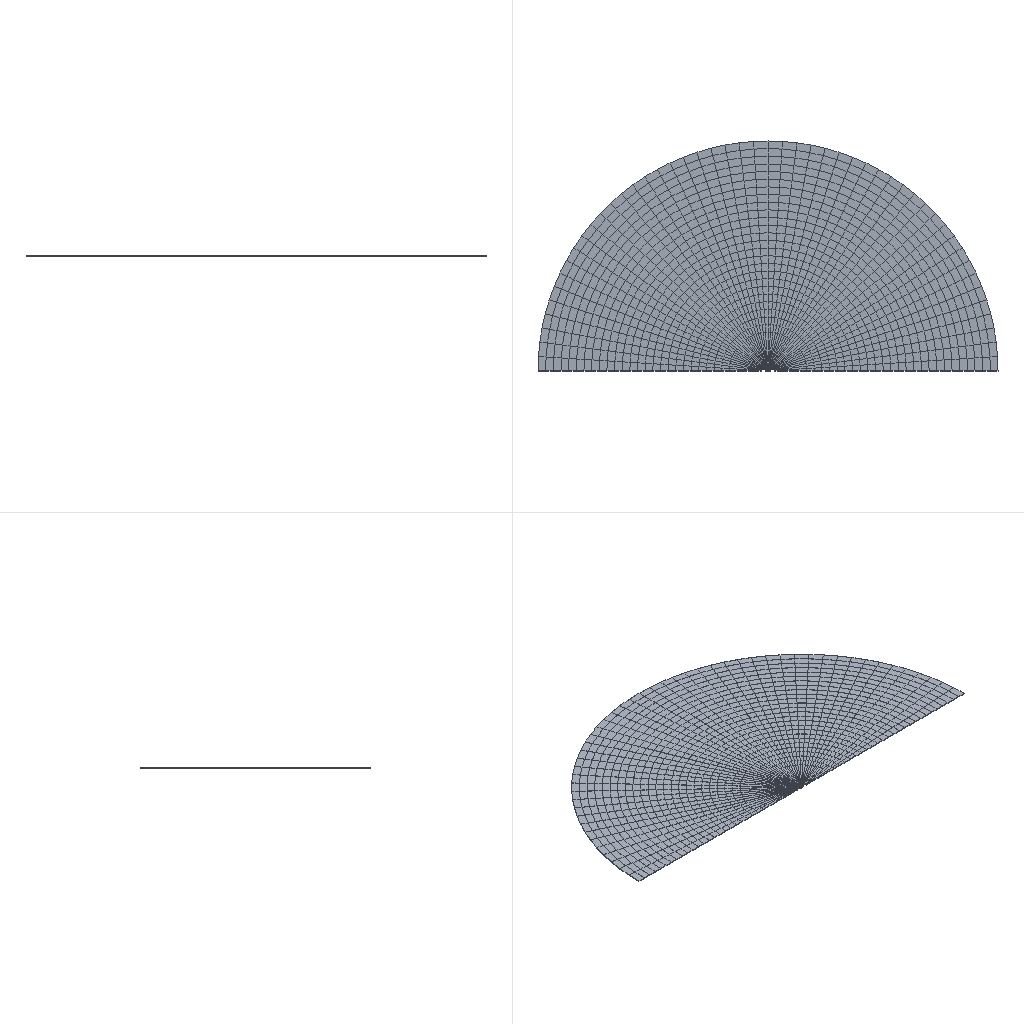Simulation study | abaqus
Set-up summary:
category,name,step,type,value,unit,region
solver,abaqus
solver,version,,,Abaqus/Standard 2020
units,not stated in the deck,,not stated
analysis,deck,,soils,soils
load_step,Step-1,Step-1,soils,nlgeom=True
contact,interactions,,,general=0 pairs=0 ties=0
load_step,requested,,,1
mesh,nodes,,,4272
mesh,elements,,,2036
element_type,C3D8PT,,solid,2036
load,load commands in deck,,count,3
bc,support commands in deck,,count,11
material,MATERIAL-1,,in results
check,setup vs results,,match,"per instance, exact: element labels, types and connectivity; labels of the nodes the elements use; coordinates of those nodes at SINGLE_PRECISION in 1 of 1 instance(s)"
Abaqus input file, long lists of numbers shortened:
*Heading
** Job name: Job-1 Model name: Model-1-30tian-1fenxibu
** Generated by: Abaqus/CAE 2020
*Preprint, echo=NO, model=NO, history=NO, contact=NO
**
** PARTS
**
*Part, name=Part-1
*Node
      1,   3.104,           0., 0.01
      2,   3.104,           0.,           0.
** (4270 more lines like these left out)
*Element, type=C3D8PT
   1,  226,  276, 1867,  495,    1,    2,   17,   72
   2,  495, 1867, 1868,  496,   72,   17,   18,   71
** (2034 more lines like these left out)
*Nset, nset=_PickedSet5, internal, generate
    1,  4272,     1
*Elset, elset=_PickedSet5, internal, generate
    1,  2036,     1
** Section: Section-1
*Solid Section, elset=_PickedSet5, material=Material-1
,
*End Part
**
**
** ASSEMBLY
**
*Assembly, name=Assembly
**
*Instance, name=Part-1-1, part=Part-1
         -3.,           0.,           0.
*End Instance
**
*Nset, nset=Set-re, instance=Part-1-1
 377, 378, 379, 380, 381, 382, 383, 384, 385, 386, 387, 388, 389, 390, 391, 392
 393, 394, 395, 396, 397, 398, 399, 400, 401, 402, 403, 404, 405, 414, 415, 416
** (2 more lines like these left out)
*Nset, nset=UPandBOTTOM, instance=Part-1-1
    1,    2,    3,    4,    5,    6,    7,    8,    9,   10,   11,   12,   13,   14,   15,   16
   17,   18,   19,   20,   21,   22,   23,   24,   25,   26,   27,   28,   29,   30,   31,   32
** (258 more lines like these left out)
*Nset, nset=leng, instance=Part-1-1
 329, 330, 331, 332, 333, 334, 335, 336, 337, 338, 339, 340, 341, 342, 343, 344
 345, 346, 347, 348, 349, 350, 351, 352, 353, 354, 355, 356, 357, 462, 463, 464
** (2 more lines like these left out)
*Nset, nset=_PickedSet14, internal, instance=Part-1-1, generate
    1,  4272,     1
*Elset, elset=_PickedSet14, internal, instance=Part-1-1, generate
    1,  2036,     1
*Nset, nset=_PickedSet15, internal, instance=Part-1-1, generate
    1,  4272,     1
*Elset, elset=_PickedSet15, internal, instance=Part-1-1, generate
    1,  2036,     1
*Nset, nset=_PickedSet16, internal, instance=Part-1-1, generate
    1,  4272,     1
*Elset, elset=_PickedSet16, internal, instance=Part-1-1, generate
    1,  2036,     1
*Nset, nset=_PickedSet22, internal, instance=Part-1-1
   3,   4,   6,   7, 129, 130, 131, 132, 133, 134, 135, 136, 137, 138, 139, 140
 141, 142, 143, 144, 145, 146, 147, 148, 149, 150, 151, 152, 153, 154, 155, 156
** (5 more lines like these left out)
*Elset, elset=_PickedSet22, internal, instance=Part-1-1, generate
   29,  1450,    29
*Nset, nset=_PickedSet27, internal, instance=Part-1-1
   1,   2,   3,   4,   5,   6,   7,   8,   9,  10,  11,  12,  13,  14,  15,  16
  17,  18,  19,  20,  21,  22,  23,  24,  25,  26,  27,  28,  29,  30,  31,  32
** (10 more lines like these left out)
*Elset, elset=_PickedSet27, internal, instance=Part-1-1
    1,    2,    3,    4,    5,    6,    7,    8,    9,   10,   11,   12,   13,   14,   15,   16
   17,   18,   19,   20,   21,   22,   23,   24,   25,   26,   27,   28,   29, 1422, 1423, 1424
** (4 more lines like these left out)
*Nset, nset=_PickedSet28, internal, instance=Part-1-1, generate
  9,  16,   1
*Elset, elset=_PickedSet28, internal, instance=Part-1-1
 1526, 1528, 1536, 1540
*Nset, nset=_PickedSet29, internal, instance=Part-1-1
  11,  12,  13,  14, 377, 378, 379, 380, 381, 382, 383, 384, 385, 386, 387, 388
 389, 390, 391, 392, 393, 394, 395, 396, 397, 398, 399, 400, 401, 402, 403, 404
** (2 more lines like these left out)
*Elset, elset=_PickedSet29, internal, instance=Part-1-1
 1452, 1459, 1496, 1536, 1540, 1541, 1542, 1544, 1547, 1551, 1552, 1553, 1555, 1557, 1559, 1562
 1564, 1565, 1571, 1578, 1583, 1584, 1671, 1675, 1677, 1714, 1715, 1717, 1719, 1732
*Nset, nset=_PickedSet30, internal, instance=Part-1-1
   9,  10,  15,  16, 329, 330, 331, 332, 333, 334, 335, 336, 337, 338, 339, 340
 341, 342, 343, 344, 345, 346, 347, 348, 349, 350, 351, 352, 353, 354, 355, 356
** (2 more lines like these left out)
*Elset, elset=_PickedSet30, internal, instance=Part-1-1
 1470, 1472, 1479, 1485, 1487, 1526, 1528, 1529, 1531, 1532, 1535, 1548, 1549, 1550, 1554, 1556
 1558, 1586, 1590, 1593, 1658, 1666, 1667, 1723, 1736, 1737, 1739, 1740, 1742, 1744
*Nset, nset=_PickedSet51, internal, instance=Part-1-1
   3,   4,   6,   7, 129, 130, 131, 132, 133, 134, 135, 136, 137, 138, 139, 140
 141, 142, 143, 144, 145, 146, 147, 148, 149, 150, 151, 152, 153, 154, 155, 156
** (5 more lines like these left out)
*Elset, elset=_PickedSet51, internal, instance=Part-1-1, generate
   29,  1450,    29
*Nset, nset="_T-Datum csys-2", internal
_PickedSet22,
_PickedSet27,
** (2 more lines like these left out)
*Transform, nset="_T-Datum csys-2", type=C
          0.,           0.,           0.,           0.,           0.,           1.
*Nset, nset="_T-Datum csys-LEFT", internal
Set-re,
*Transform, nset="_T-Datum csys-LEFT", type=C
-0.06,           0.,           0., -0.06,           0.,           1.
*Nset, nset="_T-Datum csys-RIGHT", internal
leng,
*Transform, nset="_T-Datum csys-RIGHT", type=C
0.06,           0.,           0., 0.06,           0.,           1.
*End Assembly
*Amplitude, name=Amp-75
             0.,             15.,           7200.,             75.,        2592000.,             75.
*Amplitude, name=Amp-80
             0.,             15.,           7200.,             80.,        2592000.,             80.
**
** MATERIALS
**
*Material, name=Material-1
*Conductivity
3.,
*Density
1900.,
*Elastic
 1e+07, 0.3
*Expansion
 5e-07,
*Permeability, specific=9800.
 6.45e-09,2.
*Permeability, Type=SATURATION
 0.2739, 0.08001
 0.2915, 0.08002
 0.3109, 0.08002
 0.3321, 0.08003
 0.3553, 0.08003
 0.3808, 0.08004
 0.4088, 0.08005
 0.4396, 0.08006
 0.4733, 0.08009
 0.5103, 0.08012
 0.5506, 0.08016
 0.5944, 0.08024
 0.6417,  0.08035
 0.692, 0.08057
 0.7449,  0.08097
  0.7992, 0.08184
 0.8533, 0.084
 0.9046, 0.09087
 0.9498,  0.1233
 0.984,  0.4099
       1.,        1.
*Expansion, Pore Fluid, zero=4.
 2.85273e-05, 15.
 3.45619e-05, 25.
 3.71462e-05, 30.
 3.95742e-05, 35.
 4.25222e-05, 40.
    4.48e-05, 45.
 4.70391e-05, 50.
 4.91725e-05, 55.
 5.12286e-05, 60.
 5.32426e-05, 65.
 5.51788e-05, 70.
 5.70676e-05, 75.
 5.89316e-05, 80.
 6.07506e-05, 85.
 6.25442e-05, 90.
 6.42945e-05, 95.
 6.60292e-05,100.
*Sorption
-400000., 0.08001
-380000., 0.08002
-360000., 0.08002
-340000., 0.08003
-320000., 0.08003
-300000., 0.08004
-280000., 0.08005
-260000., 0.08006
-240000., 0.08009
-220000., 0.08012
-200000., 0.08016
-180000., 0.08024
-160000.,  0.08035
-140000., 0.08057
-120000.,  0.08097
-100000., 0.08184
 -80000., 0.084
 -60000., 0.09087
 -40000.,  0.1233
 -20000.,  0.4099
      0.,        1.
*Specific Heat
1210.,
**
** PHYSICAL CONSTANTS
**
*Physical Constants, absolute zero=-273., stefan boltzmann=5.67e-08
**
** BOUNDARY CONDITIONS
**
** Name: BC-1 Type: 位移/转角
*Boundary
_PickedSet22, 1, 1
** Name: BC-2 Type: 对称/反对称/完全固定
*Boundary
_PickedSet27, YSYMM
** Name: BC-3 Type: 位移/转角
*Boundary
Set-re, 1, 1
Set-re, 3, 3
** Name: BC-4 Type: 位移/转角
*Boundary
leng, 1, 1
leng, 3, 3
** Name: BC-5 Type: 位移/转角
*Boundary
_PickedSet28, 1, 1
** Name: BC-8 Type: 位移/转角
*Boundary
UPandBOTTOM, 3, 3
**
** PREDEFINED FIELDS
**
** Name: Predefined Field-1   Type: Temperature
*Initial Conditions, type=TEMPERATURE
_PickedSet14, 15.
** Name: Predefined Field-2   Type: Void ratio
*Initial Conditions, TYPE=RATIO
_PickedSet15, 0.015
** Name: Predefined Field-3   Type: Pore pressure
*Initial Conditions, TYPE=PORE PRESSURE
_PickedSet16, -16000.
** ----------------------------------------------------------------
**
** STEP: Step-1
**
*Step, name=Step-1, nlgeom=YES, inc=1000, unsymm=YES
*Soils, consolidation, end=PERIOD, utol=1e+09, creep=none, stabilize=0.0002, allsdtol=0.05, continue=NO
1., 2.592e+06, 1e-20, 25920.,
**
** BOUNDARY CONDITIONS
**
** Name: BC-6 Type: 温度
*Boundary, amplitude=Amp-80
_PickedSet29, 11, 11, 1.
** Name: BC-7 Type: 温度
*Boundary, amplitude=Amp-75
_PickedSet30, 11, 11, 1.
** Name: BC-9 Type: 温度
*Boundary
_PickedSet51, 11, 11, 15.
**
** OUTPUT REQUESTS
**
*Restart, write, frequency=0
**
** FIELD OUTPUT: F-Output-1
**
*Output, field, time interval=86400.
*Node Output
CF, NT, POR, RF, U
*Element Output, directions=YES
ELEDEN, ELEN, ENER, FLUVR, FLVEL, LE, S, SAT, TEMP, VOIDR
*Contact Output
PFL, PFLA, PTL, PTLA
**
** HISTORY OUTPUT: H-Output-1
**
*Output, history, variable=PRESELECT, time interval=86400.
*End Step
Results summary:
result,step,,completed,increments=144 time=2592000.0/2592000.0
result,analysis,,,"soils, consolidation"
result,last_loadstep,,,1
result,analysis steps,,count,1
result,primary field,,,"U, POR"
result,reaction total,,FX,0.0,model units
result,reaction total,,FY,1.2e-05,model units
result,reaction total,,FZ,1e-05,model units